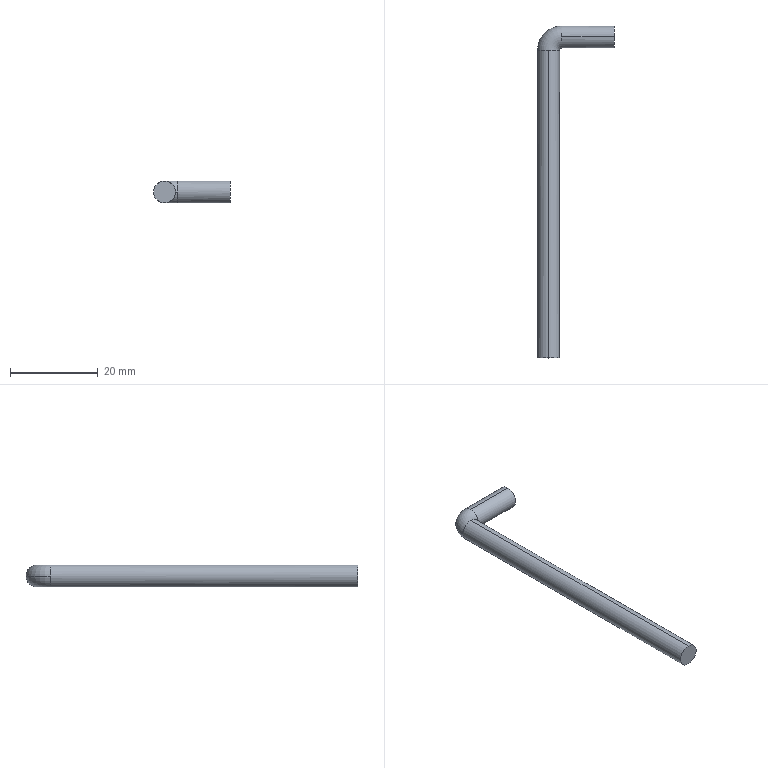Part | SolidWorks | features Sweep 1 | 1 solid | 8 faces | box 17.5 x 75.5 x 5 mm | volume 1703 mm3 | cylinder 4 | torus 2 | plane 2 | commonest cylinder face diameters 5 x4
STEP:
#1=CARTESIAN_POINT('',(0.,70.,-2.5));
#2=VERTEX_POINT('',#1);
#3=CARTESIAN_POINT('',(-2.5,70.,0.));
#4=VERTEX_POINT('',#3);
#5=CARTESIAN_POINT('',(0.,70.,0.));
#6=DIRECTION('',(0.,1.,0.));
#7=DIRECTION('',(0.,0.,1.));
#8=AXIS2_PLACEMENT_3D('',#5,#6,#7);
#9=CIRCLE('',#8,2.5);
#10=EDGE_CURVE('',#2,#4,#9,.T.);
#11=ORIENTED_EDGE('',*,*,#10,.T.);
#12=CARTESIAN_POINT('',(3.,75.5,0.));
#13=VERTEX_POINT('',#12);
#14=CARTESIAN_POINT('',(3.,70.,0.));
#15=DIRECTION('',(0.,0.,-1.));
#16=DIRECTION('',(-1.,0.,0.));
#17=AXIS2_PLACEMENT_3D('',#14,#15,#16);
#18=CIRCLE('',#17,5.5);
#19=EDGE_CURVE('',#4,#13,#18,.T.);
#20=ORIENTED_EDGE('',*,*,#19,.T.);
#21=CARTESIAN_POINT('',(3.,73.,-2.5));
#22=VERTEX_POINT('',#21);
#23=CARTESIAN_POINT('',(3.,73.,0.));
#24=DIRECTION('',(1.,0.,0.));
#25=DIRECTION('',(0.,0.,1.));
#26=AXIS2_PLACEMENT_3D('',#23,#24,#25);
#27=CIRCLE('',#26,2.5);
#28=EDGE_CURVE('',#22,#13,#27,.T.);
#29=ORIENTED_EDGE('',*,*,#28,.F.);
#30=CARTESIAN_POINT('',(3.,70.5,0.));
#31=VERTEX_POINT('',#30);
#32=CARTESIAN_POINT('',(3.,73.,0.));
#33=DIRECTION('',(1.,0.,0.));
#34=DIRECTION('',(0.,0.,1.));
#35=AXIS2_PLACEMENT_3D('',#32,#33,#34);
#36=CIRCLE('',#35,2.5);
#37=EDGE_CURVE('',#31,#22,#36,.T.);
#38=ORIENTED_EDGE('',*,*,#37,.F.);
#39=CARTESIAN_POINT('',(2.5,70.,0.));
#40=VERTEX_POINT('',#39);
#41=CARTESIAN_POINT('',(3.,70.,0.));
#42=DIRECTION('',(0.,0.,-1.));
#43=DIRECTION('',(-1.,0.,0.));
#44=AXIS2_PLACEMENT_3D('',#41,#42,#43);
#45=CIRCLE('',#44,0.5);
#46=EDGE_CURVE('',#40,#31,#45,.T.);
#47=ORIENTED_EDGE('',*,*,#46,.F.);
#48=CARTESIAN_POINT('',(0.,70.,0.));
#49=DIRECTION('',(0.,1.,0.));
#50=DIRECTION('',(0.,0.,1.));
#51=AXIS2_PLACEMENT_3D('',#48,#49,#50);
#52=CIRCLE('',#51,2.5);
#53=EDGE_CURVE('',#40,#2,#52,.T.);
#54=ORIENTED_EDGE('',*,*,#53,.T.);
#55=EDGE_LOOP('',(#11,#20,#29,#38,#47,#54));
#56=FACE_OUTER_BOUND('',#55,.T.);
#57=CARTESIAN_POINT('',(3.,70.,0.));
#58=DIRECTION('',(0.,0.,-1.));
#59=DIRECTION('',(-1.,0.,0.));
#60=AXIS2_PLACEMENT_3D('',#57,#58,#59);
#61=TOROIDAL_SURFACE('',#60,3.,2.5);
#62=ADVANCED_FACE('',(#56),#61,.T.);
#63=CARTESIAN_POINT('',(0.,70.,2.5));
#64=VERTEX_POINT('',#63);
#65=CARTESIAN_POINT('',(0.,70.,0.));
#66=DIRECTION('',(0.,1.,0.));
#67=DIRECTION('',(0.,0.,1.));
#68=AXIS2_PLACEMENT_3D('',#65,#66,#67);
#69=CIRCLE('',#68,2.5);
#70=EDGE_CURVE('',#64,#40,#69,.T.);
#71=ORIENTED_EDGE('',*,*,#70,.F.);
#72=CARTESIAN_POINT('',(0.,0.,2.5));
#73=VERTEX_POINT('',#72);
#74=CARTESIAN_POINT('',(0.,70.,2.5));
#75=DIRECTION('',(0.,-1.,0.));
#76=VECTOR('',#75,1000.);
#77=LINE('',#74,#76);
#78=EDGE_CURVE('',#64,#73,#77,.T.);
#79=ORIENTED_EDGE('',*,*,#78,.T.);
#80=CARTESIAN_POINT('',(0.,0.,-2.5));
#81=VERTEX_POINT('',#80);
#82=CARTESIAN_POINT('',(0.,0.,0.));
#83=DIRECTION('',(0.,1.,0.));
#84=DIRECTION('',(0.,0.,1.));
#85=AXIS2_PLACEMENT_3D('',#82,#83,#84);
#86=CIRCLE('',#85,2.5);
#87=EDGE_CURVE('',#73,#81,#86,.T.);
#88=ORIENTED_EDGE('',*,*,#87,.T.);
#89=CARTESIAN_POINT('',(0.,70.,-2.5));
#90=DIRECTION('',(0.,-1.,0.));
#91=VECTOR('',#90,1000.);
#92=LINE('',#89,#91);
#93=EDGE_CURVE('',#2,#81,#92,.T.);
#94=ORIENTED_EDGE('',*,*,#93,.F.);
#95=ORIENTED_EDGE('',*,*,#53,.F.);
#96=EDGE_LOOP('',(#71,#79,#88,#94,#95));
#97=FACE_OUTER_BOUND('',#96,.T.);
#98=CARTESIAN_POINT('',(0.,70.,0.));
#99=DIRECTION('',(0.,-1.,0.));
#100=DIRECTION('',(0.,0.,-1.));
#101=AXIS2_PLACEMENT_3D('',#98,#99,#100);
#102=CYLINDRICAL_SURFACE('',#101,2.5);
#103=ADVANCED_FACE('',(#97),#102,.T.);
#104=ORIENTED_EDGE('',*,*,#28,.T.);
#105=CARTESIAN_POINT('',(3.,73.,2.5));
#106=VERTEX_POINT('',#105);
#107=CARTESIAN_POINT('',(3.,73.,0.));
#108=DIRECTION('',(1.,0.,0.));
#109=DIRECTION('',(0.,0.,1.));
#110=AXIS2_PLACEMENT_3D('',#107,#108,#109);
#111=CIRCLE('',#110,2.5);
#112=EDGE_CURVE('',#13,#106,#111,.T.);
#113=ORIENTED_EDGE('',*,*,#112,.T.);
#114=CARTESIAN_POINT('',(15.,73.,2.5));
#115=VERTEX_POINT('',#114);
#116=CARTESIAN_POINT('',(3.,73.,2.5));
#117=DIRECTION('',(1.,0.,0.));
#118=VECTOR('',#117,1000.);
#119=LINE('',#116,#118);
#120=EDGE_CURVE('',#106,#115,#119,.T.);
#121=ORIENTED_EDGE('',*,*,#120,.T.);
#122=CARTESIAN_POINT('',(15.,73.,-2.5));
#123=VERTEX_POINT('',#122);
#124=CARTESIAN_POINT('',(15.,73.,0.));
#125=DIRECTION('',(1.,0.,0.));
#126=DIRECTION('',(0.,0.,1.));
#127=AXIS2_PLACEMENT_3D('',#124,#125,#126);
#128=CIRCLE('',#127,2.5);
#129=EDGE_CURVE('',#123,#115,#128,.T.);
#130=ORIENTED_EDGE('',*,*,#129,.F.);
#131=CARTESIAN_POINT('',(3.,73.,-2.5));
#132=DIRECTION('',(1.,0.,0.));
#133=VECTOR('',#132,1000.);
#134=LINE('',#131,#133);
#135=EDGE_CURVE('',#22,#123,#134,.T.);
#136=ORIENTED_EDGE('',*,*,#135,.F.);
#137=EDGE_LOOP('',(#104,#113,#121,#130,#136));
#138=FACE_OUTER_BOUND('',#137,.T.);
#139=CARTESIAN_POINT('',(3.,73.,0.));
#140=DIRECTION('',(1.,0.,0.));
#141=DIRECTION('',(0.,0.,-1.));
#142=AXIS2_PLACEMENT_3D('',#139,#140,#141);
#143=CYLINDRICAL_SURFACE('',#142,2.5);
#144=ADVANCED_FACE('',(#138),#143,.T.);
#145=ORIENTED_EDGE('',*,*,#120,.F.);
#146=CARTESIAN_POINT('',(3.,73.,0.));
#147=DIRECTION('',(1.,0.,0.));
#148=DIRECTION('',(0.,0.,1.));
#149=AXIS2_PLACEMENT_3D('',#146,#147,#148);
#150=CIRCLE('',#149,2.5);
#151=EDGE_CURVE('',#106,#31,#150,.T.);
#152=ORIENTED_EDGE('',*,*,#151,.T.);
#153=ORIENTED_EDGE('',*,*,#37,.T.);
#154=ORIENTED_EDGE('',*,*,#135,.T.);
#155=CARTESIAN_POINT('',(15.,73.,0.));
#156=DIRECTION('',(1.,0.,0.));
#157=DIRECTION('',(0.,0.,1.));
#158=AXIS2_PLACEMENT_3D('',#155,#156,#157);
#159=CIRCLE('',#158,2.5);
#160=EDGE_CURVE('',#115,#123,#159,.T.);
#161=ORIENTED_EDGE('',*,*,#160,.F.);
#162=EDGE_LOOP('',(#145,#152,#153,#154,#161));
#163=FACE_OUTER_BOUND('',#162,.T.);
#164=CARTESIAN_POINT('',(3.,73.,0.));
#165=DIRECTION('',(1.,0.,0.));
#166=DIRECTION('',(0.,0.,-1.));
#167=AXIS2_PLACEMENT_3D('',#164,#165,#166);
#168=CYLINDRICAL_SURFACE('',#167,2.5);
#169=ADVANCED_FACE('',(#163),#168,.T.);
#170=ORIENTED_EDGE('',*,*,#19,.F.);
#171=CARTESIAN_POINT('',(0.,70.,0.));
#172=DIRECTION('',(0.,1.,0.));
#173=DIRECTION('',(0.,0.,1.));
#174=AXIS2_PLACEMENT_3D('',#171,#172,#173);
#175=CIRCLE('',#174,2.5);
#176=EDGE_CURVE('',#4,#64,#175,.T.);
#177=ORIENTED_EDGE('',*,*,#176,.T.);
#178=ORIENTED_EDGE('',*,*,#70,.T.);
#179=ORIENTED_EDGE('',*,*,#46,.T.);
#180=ORIENTED_EDGE('',*,*,#151,.F.);
#181=ORIENTED_EDGE('',*,*,#112,.F.);
#182=EDGE_LOOP('',(#170,#177,#178,#179,#180,#181));
#183=FACE_OUTER_BOUND('',#182,.T.);
#184=CARTESIAN_POINT('',(3.,70.,0.));
#185=DIRECTION('',(0.,0.,-1.));
#186=DIRECTION('',(-1.,0.,0.));
#187=AXIS2_PLACEMENT_3D('',#184,#185,#186);
#188=TOROIDAL_SURFACE('',#187,3.,2.5);
#189=ADVANCED_FACE('',(#183),#188,.T.);
#190=ORIENTED_EDGE('',*,*,#78,.F.);
#191=ORIENTED_EDGE('',*,*,#176,.F.);
#192=ORIENTED_EDGE('',*,*,#10,.F.);
#193=ORIENTED_EDGE('',*,*,#93,.T.);
#194=CARTESIAN_POINT('',(0.,0.,0.));
#195=DIRECTION('',(0.,1.,0.));
#196=DIRECTION('',(0.,0.,1.));
#197=AXIS2_PLACEMENT_3D('',#194,#195,#196);
#198=CIRCLE('',#197,2.5);
#199=EDGE_CURVE('',#81,#73,#198,.T.);
#200=ORIENTED_EDGE('',*,*,#199,.T.);
#201=EDGE_LOOP('',(#190,#191,#192,#193,#200));
#202=FACE_OUTER_BOUND('',#201,.T.);
#203=CARTESIAN_POINT('',(0.,70.,0.));
#204=DIRECTION('',(0.,-1.,0.));
#205=DIRECTION('',(0.,0.,-1.));
#206=AXIS2_PLACEMENT_3D('',#203,#204,#205);
#207=CYLINDRICAL_SURFACE('',#206,2.5);
#208=ADVANCED_FACE('',(#202),#207,.T.);
#209=ORIENTED_EDGE('',*,*,#129,.T.);
#210=ORIENTED_EDGE('',*,*,#160,.T.);
#211=EDGE_LOOP('',(#209,#210));
#212=FACE_OUTER_BOUND('',#211,.T.);
#213=CARTESIAN_POINT('',(15.,73.,0.));
#214=DIRECTION('',(1.,0.,0.));
#215=DIRECTION('',(0.,0.,1.));
#216=AXIS2_PLACEMENT_3D('',#213,#214,#215);
#217=PLANE('',#216);
#218=ADVANCED_FACE('',(#212),#217,.T.);
#219=ORIENTED_EDGE('',*,*,#199,.F.);
#220=ORIENTED_EDGE('',*,*,#87,.F.);
#221=EDGE_LOOP('',(#219,#220));
#222=FACE_OUTER_BOUND('',#221,.T.);
#223=CARTESIAN_POINT('',(0.,0.,0.));
#224=DIRECTION('',(0.,1.,0.));
#225=DIRECTION('',(0.,0.,1.));
#226=AXIS2_PLACEMENT_3D('',#223,#224,#225);
#227=PLANE('',#226);
#228=ADVANCED_FACE('',(#222),#227,.F.);
#229=CLOSED_SHELL('',(#62,#103,#144,#169,#189,#208,#218,#228));
#230=MANIFOLD_SOLID_BREP('',#229);
#231=CARTESIAN_POINT('',(0.,0.,0.));
#232=DIRECTION('',(0.,0.,1.));
#233=DIRECTION('',(1.,0.,0.));
#234=AXIS2_PLACEMENT_3D('',#231,#232,#233);
#235=(LENGTH_UNIT()NAMED_UNIT(*)SI_UNIT(.MILLI.,.METRE.));
#236=UNCERTAINTY_MEASURE_WITH_UNIT(LENGTH_MEASURE(0.00001),#235,'','');
#237=(NAMED_UNIT(*)PLANE_ANGLE_UNIT()SI_UNIT($,.RADIAN.));
#238=(NAMED_UNIT(*)SI_UNIT($,.STERADIAN.)SOLID_ANGLE_UNIT());
#239=(GEOMETRIC_REPRESENTATION_CONTEXT(3)GLOBAL_UNCERTAINTY_ASSIGNED_CONTEXT((#236))GLOBAL_UNIT_ASSIGNED_CONTEXT((#235,#237,#238))REPRESENTATION_CONTEXT('',''));
#240=ADVANCED_BREP_SHAPE_REPRESENTATION('',(#230,#234),#239);